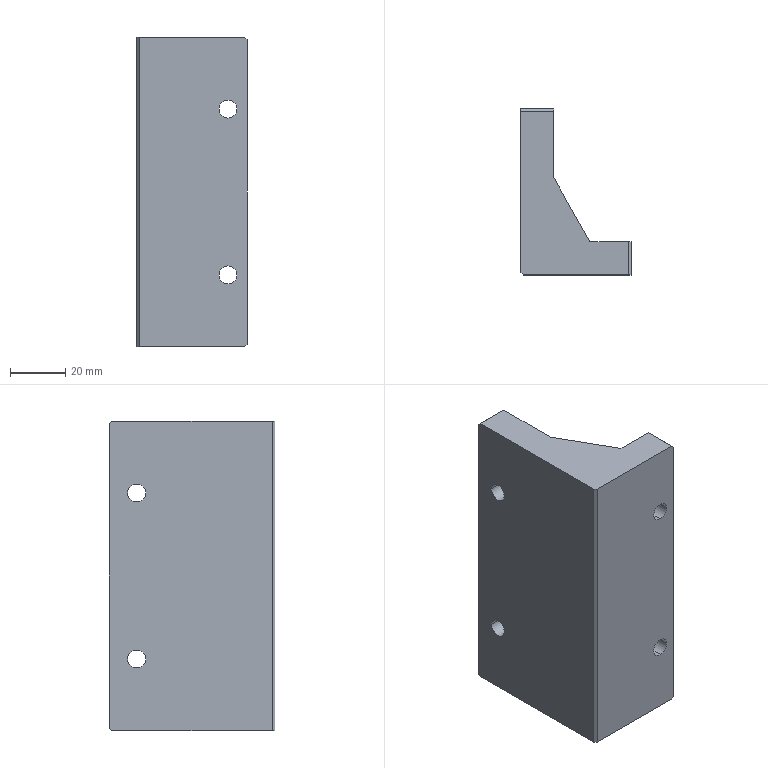Part | NX | features BREP 1 | 1 solid | 34 faces | box 40 x 60 x 112 mm | volume 133076 mm3 | cylinder 14 | plane 14 | cone 6 | commonest cylinder face diameters 6.5 x8 3.3 x6
STEP:
#1=CARTESIAN_POINT('',(9.65,10.,10.1));
#2=VERTEX_POINT('',#1);
#3=CARTESIAN_POINT('',(6.35,10.,10.1));
#4=VERTEX_POINT('',#3);
#5=CARTESIAN_POINT('',(8.,10.,10.1));
#6=DIRECTION('',(0.,0.,-1.));
#7=DIRECTION('',(-1.,0.,0.));
#8=AXIS2_PLACEMENT_3D('',#5,#6,#7);
#9=CIRCLE('',#8,1.65);
#10=EDGE_CURVE('',#2,#4,#9,.T.);
#11=ORIENTED_EDGE('',*,*,#10,.F.);
#12=CARTESIAN_POINT('',(9.65,10.,0.));
#13=VERTEX_POINT('',#12);
#14=CARTESIAN_POINT('',(9.65,10.,0.));
#15=DIRECTION('',(0.,0.,-1.));
#16=VECTOR('',#15,1000.);
#17=LINE('',#14,#16);
#18=EDGE_CURVE('',#2,#13,#17,.T.);
#19=ORIENTED_EDGE('',*,*,#18,.T.);
#20=CARTESIAN_POINT('',(6.35,10.,0.));
#21=VERTEX_POINT('',#20);
#22=CARTESIAN_POINT('',(8.,10.,0.));
#23=DIRECTION('',(0.,0.,-1.));
#24=DIRECTION('',(-1.,0.,0.));
#25=AXIS2_PLACEMENT_3D('',#22,#23,#24);
#26=CIRCLE('',#25,1.65);
#27=EDGE_CURVE('',#13,#21,#26,.T.);
#28=ORIENTED_EDGE('',*,*,#27,.T.);
#29=CARTESIAN_POINT('',(6.35,10.,0.));
#30=DIRECTION('',(0.,0.,-1.));
#31=VECTOR('',#30,1000.);
#32=LINE('',#29,#31);
#33=EDGE_CURVE('',#4,#21,#32,.T.);
#34=ORIENTED_EDGE('',*,*,#33,.F.);
#35=EDGE_LOOP('',(#11,#19,#28,#34));
#36=FACE_BOUND('',#35,.T.);
#37=CARTESIAN_POINT('',(8.,10.,0.));
#38=DIRECTION('',(0.,0.,-1.));
#39=DIRECTION('',(-1.,0.,0.));
#40=AXIS2_PLACEMENT_3D('',#37,#38,#39);
#41=CYLINDRICAL_SURFACE('',#40,1.65);
#42=ADVANCED_FACE('',(#36),#41,.F.);
#43=CARTESIAN_POINT('',(8.,10.,11.091));
#44=VERTEX_POINT('',#43);
#45=CARTESIAN_POINT('',(6.35,10.,10.1));
#46=DIRECTION('',(-0.8572,0.,-0.515));
#47=VECTOR('',#46,1000.);
#48=LINE('',#45,#47);
#49=EDGE_CURVE('',#44,#4,#48,.T.);
#50=ORIENTED_EDGE('',*,*,#49,.F.);
#51=CARTESIAN_POINT('',(9.65,10.,10.1));
#52=DIRECTION('',(0.8572,0.,-0.515));
#53=VECTOR('',#52,1000.);
#54=LINE('',#51,#53);
#55=EDGE_CURVE('',#44,#2,#54,.T.);
#56=ORIENTED_EDGE('',*,*,#55,.T.);
#57=ORIENTED_EDGE('',*,*,#10,.T.);
#58=EDGE_LOOP('',(#50,#56,#57));
#59=FACE_BOUND('',#58,.T.);
#60=CARTESIAN_POINT('',(8.,10.,10.1));
#61=DIRECTION('',(0.,0.,-1.));
#62=DIRECTION('',(-1.,0.,0.));
#63=AXIS2_PLACEMENT_3D('',#60,#61,#62);
#64=CONICAL_SURFACE('',#63,1.65,1.03);
#65=ADVANCED_FACE('',(#59),#64,.F.);
#66=CARTESIAN_POINT('',(8.,49.9,94.35));
#67=VERTEX_POINT('',#66);
#68=CARTESIAN_POINT('',(8.,49.9,97.65));
#69=VERTEX_POINT('',#68);
#70=CARTESIAN_POINT('',(8.,49.9,96.));
#71=DIRECTION('',(0.,1.,0.));
#72=DIRECTION('',(0.,0.,1.));
#73=AXIS2_PLACEMENT_3D('',#70,#71,#72);
#74=CIRCLE('',#73,1.65);
#75=EDGE_CURVE('',#67,#69,#74,.T.);
#76=ORIENTED_EDGE('',*,*,#75,.F.);
#77=CARTESIAN_POINT('',(8.,60.,94.35));
#78=VERTEX_POINT('',#77);
#79=CARTESIAN_POINT('',(8.,60.,94.35));
#80=DIRECTION('',(0.,1.,0.));
#81=VECTOR('',#80,1000.);
#82=LINE('',#79,#81);
#83=EDGE_CURVE('',#78,#67,#82,.F.);
#84=ORIENTED_EDGE('',*,*,#83,.F.);
#85=CARTESIAN_POINT('',(8.,60.,97.65));
#86=VERTEX_POINT('',#85);
#87=CARTESIAN_POINT('',(8.,60.,96.));
#88=DIRECTION('',(0.,1.,0.));
#89=DIRECTION('',(0.,0.,1.));
#90=AXIS2_PLACEMENT_3D('',#87,#88,#89);
#91=CIRCLE('',#90,1.65);
#92=EDGE_CURVE('',#78,#86,#91,.T.);
#93=ORIENTED_EDGE('',*,*,#92,.T.);
#94=CARTESIAN_POINT('',(8.,60.,97.65));
#95=DIRECTION('',(0.,1.,0.));
#96=VECTOR('',#95,1000.);
#97=LINE('',#94,#96);
#98=EDGE_CURVE('',#86,#69,#97,.F.);
#99=ORIENTED_EDGE('',*,*,#98,.T.);
#100=EDGE_LOOP('',(#76,#84,#93,#99));
#101=FACE_BOUND('',#100,.T.);
#102=CARTESIAN_POINT('',(8.,60.,96.));
#103=DIRECTION('',(0.,1.,0.));
#104=DIRECTION('',(0.,0.,1.));
#105=AXIS2_PLACEMENT_3D('',#102,#103,#104);
#106=CYLINDRICAL_SURFACE('',#105,1.65);
#107=ADVANCED_FACE('',(#101),#106,.F.);
#108=CARTESIAN_POINT('',(8.,48.909,96.));
#109=VERTEX_POINT('',#108);
#110=CARTESIAN_POINT('',(8.,49.9,97.65));
#111=DIRECTION('',(0.,0.515,0.8572));
#112=VECTOR('',#111,1000.);
#113=LINE('',#110,#112);
#114=EDGE_CURVE('',#69,#109,#113,.F.);
#115=ORIENTED_EDGE('',*,*,#114,.T.);
#116=CARTESIAN_POINT('',(8.,49.9,94.35));
#117=DIRECTION('',(0.,0.515,-0.8572));
#118=VECTOR('',#117,1000.);
#119=LINE('',#116,#118);
#120=EDGE_CURVE('',#67,#109,#119,.F.);
#121=ORIENTED_EDGE('',*,*,#120,.F.);
#122=ORIENTED_EDGE('',*,*,#75,.T.);
#123=EDGE_LOOP('',(#115,#121,#122));
#124=FACE_BOUND('',#123,.T.);
#125=CARTESIAN_POINT('',(8.,49.9,96.));
#126=DIRECTION('',(0.,1.,0.));
#127=DIRECTION('',(0.,0.,1.));
#128=AXIS2_PLACEMENT_3D('',#125,#126,#127);
#129=CONICAL_SURFACE('',#128,1.65,1.03);
#130=ADVANCED_FACE('',(#124),#129,.F.);
#131=CARTESIAN_POINT('',(8.,49.9,14.35));
#132=VERTEX_POINT('',#131);
#133=CARTESIAN_POINT('',(8.,49.9,17.65));
#134=VERTEX_POINT('',#133);
#135=CARTESIAN_POINT('',(8.,49.9,16.));
#136=DIRECTION('',(0.,1.,0.));
#137=DIRECTION('',(0.,0.,1.));
#138=AXIS2_PLACEMENT_3D('',#135,#136,#137);
#139=CIRCLE('',#138,1.65);
#140=EDGE_CURVE('',#132,#134,#139,.T.);
#141=ORIENTED_EDGE('',*,*,#140,.F.);
#142=CARTESIAN_POINT('',(8.,60.,14.35));
#143=VERTEX_POINT('',#142);
#144=CARTESIAN_POINT('',(8.,60.,14.35));
#145=DIRECTION('',(0.,1.,0.));
#146=VECTOR('',#145,1000.);
#147=LINE('',#144,#146);
#148=EDGE_CURVE('',#143,#132,#147,.F.);
#149=ORIENTED_EDGE('',*,*,#148,.F.);
#150=CARTESIAN_POINT('',(8.,60.,17.65));
#151=VERTEX_POINT('',#150);
#152=CARTESIAN_POINT('',(8.,60.,16.));
#153=DIRECTION('',(0.,1.,0.));
#154=DIRECTION('',(0.,0.,1.));
#155=AXIS2_PLACEMENT_3D('',#152,#153,#154);
#156=CIRCLE('',#155,1.65);
#157=EDGE_CURVE('',#143,#151,#156,.T.);
#158=ORIENTED_EDGE('',*,*,#157,.T.);
#159=CARTESIAN_POINT('',(8.,60.,17.65));
#160=DIRECTION('',(0.,1.,0.));
#161=VECTOR('',#160,1000.);
#162=LINE('',#159,#161);
#163=EDGE_CURVE('',#151,#134,#162,.F.);
#164=ORIENTED_EDGE('',*,*,#163,.T.);
#165=EDGE_LOOP('',(#141,#149,#158,#164));
#166=FACE_BOUND('',#165,.T.);
#167=CARTESIAN_POINT('',(8.,60.,16.));
#168=DIRECTION('',(0.,1.,0.));
#169=DIRECTION('',(0.,0.,1.));
#170=AXIS2_PLACEMENT_3D('',#167,#168,#169);
#171=CYLINDRICAL_SURFACE('',#170,1.65);
#172=ADVANCED_FACE('',(#166),#171,.F.);
#173=CARTESIAN_POINT('',(8.,48.909,16.));
#174=VERTEX_POINT('',#173);
#175=CARTESIAN_POINT('',(8.,49.9,17.65));
#176=DIRECTION('',(0.,0.515,0.8572));
#177=VECTOR('',#176,1000.);
#178=LINE('',#175,#177);
#179=EDGE_CURVE('',#134,#174,#178,.F.);
#180=ORIENTED_EDGE('',*,*,#179,.T.);
#181=CARTESIAN_POINT('',(8.,49.9,14.35));
#182=DIRECTION('',(0.,0.515,-0.8572));
#183=VECTOR('',#182,1000.);
#184=LINE('',#181,#183);
#185=EDGE_CURVE('',#132,#174,#184,.F.);
#186=ORIENTED_EDGE('',*,*,#185,.F.);
#187=ORIENTED_EDGE('',*,*,#140,.T.);
#188=EDGE_LOOP('',(#180,#186,#187));
#189=FACE_BOUND('',#188,.T.);
#190=CARTESIAN_POINT('',(8.,49.9,16.));
#191=DIRECTION('',(0.,1.,0.));
#192=DIRECTION('',(0.,0.,1.));
#193=AXIS2_PLACEMENT_3D('',#190,#191,#192);
#194=CONICAL_SURFACE('',#193,1.65,1.03);
#195=ADVANCED_FACE('',(#189),#194,.F.);
#196=CARTESIAN_POINT('',(0.,46.75,86.));
#197=VERTEX_POINT('',#196);
#198=CARTESIAN_POINT('',(0.,53.25,86.));
#199=VERTEX_POINT('',#198);
#200=CARTESIAN_POINT('',(0.,50.,86.));
#201=DIRECTION('',(1.,0.,0.));
#202=DIRECTION('',(0.,0.,-1.));
#203=AXIS2_PLACEMENT_3D('',#200,#201,#202);
#204=CIRCLE('',#203,3.25);
#205=EDGE_CURVE('',#197,#199,#204,.T.);
#206=ORIENTED_EDGE('',*,*,#205,.F.);
#207=CARTESIAN_POINT('',(12.,46.75,86.));
#208=VERTEX_POINT('',#207);
#209=CARTESIAN_POINT('',(-18.,46.75,86.));
#210=DIRECTION('',(1.,0.,0.));
#211=VECTOR('',#210,1000.);
#212=LINE('',#209,#211);
#213=EDGE_CURVE('',#208,#197,#212,.F.);
#214=ORIENTED_EDGE('',*,*,#213,.F.);
#215=CARTESIAN_POINT('',(12.,53.25,86.));
#216=VERTEX_POINT('',#215);
#217=CARTESIAN_POINT('',(12.,50.,86.));
#218=DIRECTION('',(1.,0.,0.));
#219=DIRECTION('',(0.,1.,0.));
#220=AXIS2_PLACEMENT_3D('',#217,#218,#219);
#221=CIRCLE('',#220,3.25);
#222=EDGE_CURVE('',#208,#216,#221,.T.);
#223=ORIENTED_EDGE('',*,*,#222,.T.);
#224=CARTESIAN_POINT('',(-18.,53.25,86.));
#225=DIRECTION('',(1.,0.,0.));
#226=VECTOR('',#225,1000.);
#227=LINE('',#224,#226);
#228=EDGE_CURVE('',#216,#199,#227,.F.);
#229=ORIENTED_EDGE('',*,*,#228,.T.);
#230=EDGE_LOOP('',(#206,#214,#223,#229));
#231=FACE_BOUND('',#230,.T.);
#232=CARTESIAN_POINT('',(-18.,50.,86.));
#233=DIRECTION('',(1.,0.,0.));
#234=DIRECTION('',(0.,1.,0.));
#235=AXIS2_PLACEMENT_3D('',#232,#233,#234);
#236=CYLINDRICAL_SURFACE('',#235,3.25);
#237=ADVANCED_FACE('',(#231),#236,.F.);
#238=CARTESIAN_POINT('',(0.,46.75,26.));
#239=VERTEX_POINT('',#238);
#240=CARTESIAN_POINT('',(0.,53.25,26.));
#241=VERTEX_POINT('',#240);
#242=CARTESIAN_POINT('',(0.,50.,26.));
#243=DIRECTION('',(1.,0.,0.));
#244=DIRECTION('',(0.,0.,-1.));
#245=AXIS2_PLACEMENT_3D('',#242,#243,#244);
#246=CIRCLE('',#245,3.25);
#247=EDGE_CURVE('',#239,#241,#246,.T.);
#248=ORIENTED_EDGE('',*,*,#247,.F.);
#249=CARTESIAN_POINT('',(12.,46.75,26.));
#250=VERTEX_POINT('',#249);
#251=CARTESIAN_POINT('',(-18.,46.75,26.));
#252=DIRECTION('',(1.,0.,0.));
#253=VECTOR('',#252,1000.);
#254=LINE('',#251,#253);
#255=EDGE_CURVE('',#250,#239,#254,.F.);
#256=ORIENTED_EDGE('',*,*,#255,.F.);
#257=CARTESIAN_POINT('',(12.,53.25,26.));
#258=VERTEX_POINT('',#257);
#259=CARTESIAN_POINT('',(12.,50.,26.));
#260=DIRECTION('',(1.,0.,0.));
#261=DIRECTION('',(0.,1.,0.));
#262=AXIS2_PLACEMENT_3D('',#259,#260,#261);
#263=CIRCLE('',#262,3.25);
#264=EDGE_CURVE('',#250,#258,#263,.T.);
#265=ORIENTED_EDGE('',*,*,#264,.T.);
#266=CARTESIAN_POINT('',(-18.,53.25,26.));
#267=DIRECTION('',(1.,0.,0.));
#268=VECTOR('',#267,1000.);
#269=LINE('',#266,#268);
#270=EDGE_CURVE('',#258,#241,#269,.F.);
#271=ORIENTED_EDGE('',*,*,#270,.T.);
#272=EDGE_LOOP('',(#248,#256,#265,#271));
#273=FACE_BOUND('',#272,.T.);
#274=CARTESIAN_POINT('',(-18.,50.,26.));
#275=DIRECTION('',(1.,0.,0.));
#276=DIRECTION('',(0.,1.,0.));
#277=AXIS2_PLACEMENT_3D('',#274,#275,#276);
#278=CYLINDRICAL_SURFACE('',#277,3.25);
#279=ADVANCED_FACE('',(#273),#278,.F.);
#280=CARTESIAN_POINT('',(33.,0.,22.75));
#281=VERTEX_POINT('',#280);
#282=CARTESIAN_POINT('',(33.,0.,29.25));
#283=VERTEX_POINT('',#282);
#284=CARTESIAN_POINT('',(33.,0.,26.));
#285=DIRECTION('',(0.,1.,0.));
#286=DIRECTION('',(0.,0.,1.));
#287=AXIS2_PLACEMENT_3D('',#284,#285,#286);
#288=CIRCLE('',#287,3.25);
#289=EDGE_CURVE('',#281,#283,#288,.T.);
#290=ORIENTED_EDGE('',*,*,#289,.F.);
#291=CARTESIAN_POINT('',(33.,12.,22.75));
#292=VERTEX_POINT('',#291);
#293=CARTESIAN_POINT('',(33.,12.,22.75));
#294=DIRECTION('',(0.,1.,0.));
#295=VECTOR('',#294,1000.);
#296=LINE('',#293,#295);
#297=EDGE_CURVE('',#292,#281,#296,.F.);
#298=ORIENTED_EDGE('',*,*,#297,.F.);
#299=CARTESIAN_POINT('',(33.,12.,29.25));
#300=VERTEX_POINT('',#299);
#301=CARTESIAN_POINT('',(33.,12.,26.));
#302=DIRECTION('',(0.,1.,0.));
#303=DIRECTION('',(0.,0.,1.));
#304=AXIS2_PLACEMENT_3D('',#301,#302,#303);
#305=CIRCLE('',#304,3.25);
#306=EDGE_CURVE('',#292,#300,#305,.T.);
#307=ORIENTED_EDGE('',*,*,#306,.T.);
#308=CARTESIAN_POINT('',(33.,12.,29.25));
#309=DIRECTION('',(0.,1.,0.));
#310=VECTOR('',#309,1000.);
#311=LINE('',#308,#310);
#312=EDGE_CURVE('',#300,#283,#311,.F.);
#313=ORIENTED_EDGE('',*,*,#312,.T.);
#314=EDGE_LOOP('',(#290,#298,#307,#313));
#315=FACE_BOUND('',#314,.T.);
#316=CARTESIAN_POINT('',(33.,12.,26.));
#317=DIRECTION('',(0.,1.,0.));
#318=DIRECTION('',(0.,0.,1.));
#319=AXIS2_PLACEMENT_3D('',#316,#317,#318);
#320=CYLINDRICAL_SURFACE('',#319,3.25);
#321=ADVANCED_FACE('',(#315),#320,.F.);
#322=CARTESIAN_POINT('',(33.,0.,82.75));
#323=VERTEX_POINT('',#322);
#324=CARTESIAN_POINT('',(33.,0.,89.25));
#325=VERTEX_POINT('',#324);
#326=CARTESIAN_POINT('',(33.,0.,86.));
#327=DIRECTION('',(0.,1.,0.));
#328=DIRECTION('',(0.,0.,1.));
#329=AXIS2_PLACEMENT_3D('',#326,#327,#328);
#330=CIRCLE('',#329,3.25);
#331=EDGE_CURVE('',#323,#325,#330,.T.);
#332=ORIENTED_EDGE('',*,*,#331,.F.);
#333=CARTESIAN_POINT('',(33.,12.,82.75));
#334=VERTEX_POINT('',#333);
#335=CARTESIAN_POINT('',(33.,12.,82.75));
#336=DIRECTION('',(0.,1.,0.));
#337=VECTOR('',#336,1000.);
#338=LINE('',#335,#337);
#339=EDGE_CURVE('',#334,#323,#338,.F.);
#340=ORIENTED_EDGE('',*,*,#339,.F.);
#341=CARTESIAN_POINT('',(33.,12.,89.25));
#342=VERTEX_POINT('',#341);
#343=CARTESIAN_POINT('',(33.,12.,86.));
#344=DIRECTION('',(0.,1.,0.));
#345=DIRECTION('',(0.,0.,1.));
#346=AXIS2_PLACEMENT_3D('',#343,#344,#345);
#347=CIRCLE('',#346,3.25);
#348=EDGE_CURVE('',#334,#342,#347,.T.);
#349=ORIENTED_EDGE('',*,*,#348,.T.);
#350=CARTESIAN_POINT('',(33.,12.,89.25));
#351=DIRECTION('',(0.,1.,0.));
#352=VECTOR('',#351,1000.);
#353=LINE('',#350,#352);
#354=EDGE_CURVE('',#342,#325,#353,.F.);
#355=ORIENTED_EDGE('',*,*,#354,.T.);
#356=EDGE_LOOP('',(#332,#340,#349,#355));
#357=FACE_BOUND('',#356,.T.);
#358=CARTESIAN_POINT('',(33.,12.,86.));
#359=DIRECTION('',(0.,1.,0.));
#360=DIRECTION('',(0.,0.,1.));
#361=AXIS2_PLACEMENT_3D('',#358,#359,#360);
#362=CYLINDRICAL_SURFACE('',#361,3.25);
#363=ADVANCED_FACE('',(#357),#362,.F.);
#364=CARTESIAN_POINT('',(1.,0.,112.));
#365=VERTEX_POINT('',#364);
#366=CARTESIAN_POINT('',(39.,0.,112.));
#367=VERTEX_POINT('',#366);
#368=CARTESIAN_POINT('',(40.,0.,112.));
#369=DIRECTION('',(1.,0.,0.));
#370=VECTOR('',#369,1000.);
#371=LINE('',#368,#370);
#372=EDGE_CURVE('',#365,#367,#371,.T.);
#373=ORIENTED_EDGE('',*,*,#372,.F.);
#374=CARTESIAN_POINT('',(1.,0.,0.));
#375=VERTEX_POINT('',#374);
#376=CARTESIAN_POINT('',(1.,0.,112.));
#377=DIRECTION('',(0.,0.,-1.));
#378=VECTOR('',#377,1000.);
#379=LINE('',#376,#378);
#380=EDGE_CURVE('',#365,#375,#379,.T.);
#381=ORIENTED_EDGE('',*,*,#380,.T.);
#382=CARTESIAN_POINT('',(39.,0.,0.));
#383=VERTEX_POINT('',#382);
#384=CARTESIAN_POINT('',(40.,0.,0.));
#385=DIRECTION('',(1.,0.,0.));
#386=VECTOR('',#385,1000.);
#387=LINE('',#384,#386);
#388=EDGE_CURVE('',#375,#383,#387,.T.);
#389=ORIENTED_EDGE('',*,*,#388,.T.);
#390=CARTESIAN_POINT('',(40.,0.,1.));
#391=VERTEX_POINT('',#390);
#392=CARTESIAN_POINT('',(40.,0.,1.));
#393=DIRECTION('',(0.7071,0.,0.7071));
#394=VECTOR('',#393,1000.);
#395=LINE('',#392,#394);
#396=EDGE_CURVE('',#383,#391,#395,.T.);
#397=ORIENTED_EDGE('',*,*,#396,.T.);
#398=CARTESIAN_POINT('',(40.,0.,111.));
#399=VERTEX_POINT('',#398);
#400=CARTESIAN_POINT('',(40.,0.,112.));
#401=DIRECTION('',(0.,0.,-1.));
#402=VECTOR('',#401,1000.);
#403=LINE('',#400,#402);
#404=EDGE_CURVE('',#399,#391,#403,.T.);
#405=ORIENTED_EDGE('',*,*,#404,.F.);
#406=CARTESIAN_POINT('',(39.,0.,112.));
#407=DIRECTION('',(-0.7071,0.,0.7071));
#408=VECTOR('',#407,1000.);
#409=LINE('',#406,#408);
#410=EDGE_CURVE('',#399,#367,#409,.T.);
#411=ORIENTED_EDGE('',*,*,#410,.T.);
#412=EDGE_LOOP('',(#373,#381,#389,#397,#405,#411));
#413=FACE_BOUND('',#412,.T.);
#414=CARTESIAN_POINT('',(33.,0.,26.));
#415=DIRECTION('',(0.,1.,0.));
#416=DIRECTION('',(0.,0.,1.));
#417=AXIS2_PLACEMENT_3D('',#414,#415,#416);
#418=CIRCLE('',#417,3.25);
#419=EDGE_CURVE('',#283,#281,#418,.T.);
#420=ORIENTED_EDGE('',*,*,#419,.T.);
#421=ORIENTED_EDGE('',*,*,#289,.T.);
#422=EDGE_LOOP('',(#420,#421));
#423=FACE_BOUND('',#422,.T.);
#424=CARTESIAN_POINT('',(33.,0.,86.));
#425=DIRECTION('',(0.,1.,0.));
#426=DIRECTION('',(0.,0.,1.));
#427=AXIS2_PLACEMENT_3D('',#424,#425,#426);
#428=CIRCLE('',#427,3.25);
#429=EDGE_CURVE('',#325,#323,#428,.T.);
#430=ORIENTED_EDGE('',*,*,#429,.T.);
#431=ORIENTED_EDGE('',*,*,#331,.T.);
#432=EDGE_LOOP('',(#430,#431));
#433=FACE_BOUND('',#432,.T.);
#434=CARTESIAN_POINT('',(40.,0.,112.));
#435=DIRECTION('',(0.,1.,0.));
#436=DIRECTION('',(1.,0.,0.));
#437=AXIS2_PLACEMENT_3D('',#434,#435,#436);
#438=PLANE('',#437);
#439=ADVANCED_FACE('',(#413,#423,#433),#438,.F.);
#440=ORIENTED_EDGE('',*,*,#404,.T.);
#441=CARTESIAN_POINT('',(40.,12.,1.));
#442=VERTEX_POINT('',#441);
#443=CARTESIAN_POINT('',(40.,12.,1.));
#444=DIRECTION('',(0.,1.,0.));
#445=VECTOR('',#444,1000.);
#446=LINE('',#443,#445);
#447=EDGE_CURVE('',#391,#442,#446,.T.);
#448=ORIENTED_EDGE('',*,*,#447,.T.);
#449=CARTESIAN_POINT('',(40.,12.,111.));
#450=VERTEX_POINT('',#449);
#451=CARTESIAN_POINT('',(40.,12.,112.));
#452=DIRECTION('',(0.,0.,-1.));
#453=VECTOR('',#452,1000.);
#454=LINE('',#451,#453);
#455=EDGE_CURVE('',#450,#442,#454,.T.);
#456=ORIENTED_EDGE('',*,*,#455,.F.);
#457=CARTESIAN_POINT('',(40.,12.,111.));
#458=DIRECTION('',(0.,-1.,0.));
#459=VECTOR('',#458,1000.);
#460=LINE('',#457,#459);
#461=EDGE_CURVE('',#450,#399,#460,.T.);
#462=ORIENTED_EDGE('',*,*,#461,.T.);
#463=EDGE_LOOP('',(#440,#448,#456,#462));
#464=FACE_BOUND('',#463,.T.);
#465=CARTESIAN_POINT('',(40.,12.,112.));
#466=DIRECTION('',(-1.,0.,0.));
#467=DIRECTION('',(0.,0.,1.));
#468=AXIS2_PLACEMENT_3D('',#465,#466,#467);
#469=PLANE('',#468);
#470=ADVANCED_FACE('',(#464),#469,.F.);
#471=ORIENTED_EDGE('',*,*,#455,.T.);
#472=CARTESIAN_POINT('',(39.,12.,0.));
#473=VERTEX_POINT('',#472);
#474=CARTESIAN_POINT('',(40.,12.,1.));
#475=DIRECTION('',(-0.7071,0.,-0.7071));
#476=VECTOR('',#475,1000.);
#477=LINE('',#474,#476);
#478=EDGE_CURVE('',#442,#473,#477,.T.);
#479=ORIENTED_EDGE('',*,*,#478,.T.);
#480=CARTESIAN_POINT('',(25.,12.,0.));
#481=VERTEX_POINT('',#480);
#482=CARTESIAN_POINT('',(25.,12.,0.));
#483=DIRECTION('',(-1.,0.,0.));
#484=VECTOR('',#483,1000.);
#485=LINE('',#482,#484);
#486=EDGE_CURVE('',#473,#481,#485,.T.);
#487=ORIENTED_EDGE('',*,*,#486,.T.);
#488=CARTESIAN_POINT('',(25.,12.,112.));
#489=VERTEX_POINT('',#488);
#490=CARTESIAN_POINT('',(25.,12.,112.));
#491=DIRECTION('',(0.,0.,-1.));
#492=VECTOR('',#491,1000.);
#493=LINE('',#490,#492);
#494=EDGE_CURVE('',#489,#481,#493,.T.);
#495=ORIENTED_EDGE('',*,*,#494,.F.);
#496=CARTESIAN_POINT('',(39.,12.,112.));
#497=VERTEX_POINT('',#496);
#498=CARTESIAN_POINT('',(25.,12.,112.));
#499=DIRECTION('',(-1.,0.,0.));
#500=VECTOR('',#499,1000.);
#501=LINE('',#498,#500);
#502=EDGE_CURVE('',#497,#489,#501,.T.);
#503=ORIENTED_EDGE('',*,*,#502,.F.);
#504=CARTESIAN_POINT('',(39.,12.,112.));
#505=DIRECTION('',(0.7071,0.,-0.7071));
#506=VECTOR('',#505,1000.);
#507=LINE('',#504,#506);
#508=EDGE_CURVE('',#497,#450,#507,.T.);
#509=ORIENTED_EDGE('',*,*,#508,.T.);
#510=EDGE_LOOP('',(#471,#479,#487,#495,#503,#509));
#511=FACE_BOUND('',#510,.T.);
#512=CARTESIAN_POINT('',(33.,12.,26.));
#513=DIRECTION('',(0.,1.,0.));
#514=DIRECTION('',(0.,0.,1.));
#515=AXIS2_PLACEMENT_3D('',#512,#513,#514);
#516=CIRCLE('',#515,3.25);
#517=EDGE_CURVE('',#300,#292,#516,.T.);
#518=ORIENTED_EDGE('',*,*,#517,.F.);
#519=ORIENTED_EDGE('',*,*,#306,.F.);
#520=EDGE_LOOP('',(#518,#519));
#521=FACE_BOUND('',#520,.T.);
#522=CARTESIAN_POINT('',(33.,12.,86.));
#523=DIRECTION('',(0.,1.,0.));
#524=DIRECTION('',(0.,0.,1.));
#525=AXIS2_PLACEMENT_3D('',#522,#523,#524);
#526=CIRCLE('',#525,3.25);
#527=EDGE_CURVE('',#342,#334,#526,.T.);
#528=ORIENTED_EDGE('',*,*,#527,.F.);
#529=ORIENTED_EDGE('',*,*,#348,.F.);
#530=EDGE_LOOP('',(#528,#529));
#531=FACE_BOUND('',#530,.T.);
#532=CARTESIAN_POINT('',(25.,12.,112.));
#533=DIRECTION('',(0.,-1.,0.));
#534=DIRECTION('',(0.,0.,-1.));
#535=AXIS2_PLACEMENT_3D('',#532,#533,#534);
#536=PLANE('',#535);
#537=ADVANCED_FACE('',(#511,#521,#531),#536,.F.);
#538=CARTESIAN_POINT('',(12.,35.,0.));
#539=VERTEX_POINT('',#538);
#540=CARTESIAN_POINT('',(12.,35.,0.));
#541=DIRECTION('',(-0.4921,0.8706,0.));
#542=VECTOR('',#541,1000.);
#543=LINE('',#540,#542);
#544=EDGE_CURVE('',#481,#539,#543,.T.);
#545=ORIENTED_EDGE('',*,*,#544,.T.);
#546=CARTESIAN_POINT('',(12.,35.,112.));
#547=VERTEX_POINT('',#546);
#548=CARTESIAN_POINT('',(12.,35.,112.));
#549=DIRECTION('',(0.,0.,-1.));
#550=VECTOR('',#549,1000.);
#551=LINE('',#548,#550);
#552=EDGE_CURVE('',#547,#539,#551,.T.);
#553=ORIENTED_EDGE('',*,*,#552,.F.);
#554=CARTESIAN_POINT('',(12.,35.,112.));
#555=DIRECTION('',(-0.4921,0.8706,0.));
#556=VECTOR('',#555,1000.);
#557=LINE('',#554,#556);
#558=EDGE_CURVE('',#489,#547,#557,.T.);
#559=ORIENTED_EDGE('',*,*,#558,.F.);
#560=ORIENTED_EDGE('',*,*,#494,.T.);
#561=EDGE_LOOP('',(#545,#553,#559,#560));
#562=FACE_BOUND('',#561,.T.);
#563=CARTESIAN_POINT('',(12.,35.,112.));
#564=DIRECTION('',(-0.8706,-0.4921,0.));
#565=DIRECTION('',(-0.4921,0.8706,0.));
#566=AXIS2_PLACEMENT_3D('',#563,#564,#565);
#567=PLANE('',#566);
#568=ADVANCED_FACE('',(#562),#567,.F.);
#569=CARTESIAN_POINT('',(12.,60.,111.));
#570=VERTEX_POINT('',#569);
#571=CARTESIAN_POINT('',(12.,60.,1.));
#572=VERTEX_POINT('',#571);
#573=CARTESIAN_POINT('',(12.,60.,112.));
#574=DIRECTION('',(0.,0.,-1.));
#575=VECTOR('',#574,1000.);
#576=LINE('',#573,#575);
#577=EDGE_CURVE('',#570,#572,#576,.T.);
#578=ORIENTED_EDGE('',*,*,#577,.F.);
#579=CARTESIAN_POINT('',(12.,59.,112.));
#580=VERTEX_POINT('',#579);
#581=CARTESIAN_POINT('',(12.,59.,112.));
#582=DIRECTION('',(0.,-0.7071,0.7071));
#583=VECTOR('',#582,1000.);
#584=LINE('',#581,#583);
#585=EDGE_CURVE('',#570,#580,#584,.T.);
#586=ORIENTED_EDGE('',*,*,#585,.T.);
#587=CARTESIAN_POINT('',(12.,60.,112.));
#588=DIRECTION('',(0.,1.,0.));
#589=VECTOR('',#588,1000.);
#590=LINE('',#587,#589);
#591=EDGE_CURVE('',#547,#580,#590,.T.);
#592=ORIENTED_EDGE('',*,*,#591,.F.);
#593=ORIENTED_EDGE('',*,*,#552,.T.);
#594=CARTESIAN_POINT('',(12.,59.,0.));
#595=VERTEX_POINT('',#594);
#596=CARTESIAN_POINT('',(12.,60.,0.));
#597=DIRECTION('',(0.,1.,0.));
#598=VECTOR('',#597,1000.);
#599=LINE('',#596,#598);
#600=EDGE_CURVE('',#539,#595,#599,.T.);
#601=ORIENTED_EDGE('',*,*,#600,.T.);
#602=CARTESIAN_POINT('',(12.,60.,1.));
#603=DIRECTION('',(0.,0.7071,0.7071));
#604=VECTOR('',#603,1000.);
#605=LINE('',#602,#604);
#606=EDGE_CURVE('',#595,#572,#605,.T.);
#607=ORIENTED_EDGE('',*,*,#606,.T.);
#608=EDGE_LOOP('',(#578,#586,#592,#593,#601,#607));
#609=FACE_BOUND('',#608,.T.);
#610=CARTESIAN_POINT('',(12.,50.,86.));
#611=DIRECTION('',(1.,0.,0.));
#612=DIRECTION('',(0.,1.,0.));
#613=AXIS2_PLACEMENT_3D('',#610,#611,#612);
#614=CIRCLE('',#613,3.25);
#615=EDGE_CURVE('',#216,#208,#614,.T.);
#616=ORIENTED_EDGE('',*,*,#615,.F.);
#617=ORIENTED_EDGE('',*,*,#222,.F.);
#618=EDGE_LOOP('',(#616,#617));
#619=FACE_BOUND('',#618,.T.);
#620=CARTESIAN_POINT('',(12.,50.,26.));
#621=DIRECTION('',(1.,0.,0.));
#622=DIRECTION('',(0.,1.,0.));
#623=AXIS2_PLACEMENT_3D('',#620,#621,#622);
#624=CIRCLE('',#623,3.25);
#625=EDGE_CURVE('',#258,#250,#624,.T.);
#626=ORIENTED_EDGE('',*,*,#625,.F.);
#627=ORIENTED_EDGE('',*,*,#264,.F.);
#628=EDGE_LOOP('',(#626,#627));
#629=FACE_BOUND('',#628,.T.);
#630=CARTESIAN_POINT('',(12.,60.,112.));
#631=DIRECTION('',(-1.,0.,0.));
#632=DIRECTION('',(0.,1.,0.));
#633=AXIS2_PLACEMENT_3D('',#630,#631,#632);
#634=PLANE('',#633);
#635=ADVANCED_FACE('',(#609,#619,#629),#634,.F.);
#636=CARTESIAN_POINT('',(0.,60.,111.));
#637=VERTEX_POINT('',#636);
#638=CARTESIAN_POINT('',(0.,60.,1.));
#639=VERTEX_POINT('',#638);
#640=CARTESIAN_POINT('',(0.,60.,112.));
#641=DIRECTION('',(0.,0.,-1.));
#642=VECTOR('',#641,1000.);
#643=LINE('',#640,#642);
#644=EDGE_CURVE('',#637,#639,#643,.T.);
#645=ORIENTED_EDGE('',*,*,#644,.F.);
#646=CARTESIAN_POINT('',(0.,60.,111.));
#647=DIRECTION('',(1.,0.,0.));
#648=VECTOR('',#647,1000.);
#649=LINE('',#646,#648);
#650=EDGE_CURVE('',#637,#570,#649,.T.);
#651=ORIENTED_EDGE('',*,*,#650,.T.);
#652=ORIENTED_EDGE('',*,*,#577,.T.);
#653=CARTESIAN_POINT('',(0.,60.,1.));
#654=DIRECTION('',(-1.,0.,0.));
#655=VECTOR('',#654,1000.);
#656=LINE('',#653,#655);
#657=EDGE_CURVE('',#572,#639,#656,.T.);
#658=ORIENTED_EDGE('',*,*,#657,.T.);
#659=EDGE_LOOP('',(#645,#651,#652,#658));
#660=FACE_BOUND('',#659,.T.);
#661=CARTESIAN_POINT('',(8.,60.,96.));
#662=DIRECTION('',(0.,1.,0.));
#663=DIRECTION('',(0.,0.,1.));
#664=AXIS2_PLACEMENT_3D('',#661,#662,#663);
#665=CIRCLE('',#664,1.65);
#666=EDGE_CURVE('',#86,#78,#665,.T.);
#667=ORIENTED_EDGE('',*,*,#666,.F.);
#668=ORIENTED_EDGE('',*,*,#92,.F.);
#669=EDGE_LOOP('',(#667,#668));
#670=FACE_BOUND('',#669,.T.);
#671=CARTESIAN_POINT('',(8.,60.,16.));
#672=DIRECTION('',(0.,1.,0.));
#673=DIRECTION('',(0.,0.,1.));
#674=AXIS2_PLACEMENT_3D('',#671,#672,#673);
#675=CIRCLE('',#674,1.65);
#676=EDGE_CURVE('',#151,#143,#675,.T.);
#677=ORIENTED_EDGE('',*,*,#676,.F.);
#678=ORIENTED_EDGE('',*,*,#157,.F.);
#679=EDGE_LOOP('',(#677,#678));
#680=FACE_BOUND('',#679,.T.);
#681=CARTESIAN_POINT('',(0.,60.,112.));
#682=DIRECTION('',(0.,-1.,0.));
#683=DIRECTION('',(0.,0.,-1.));
#684=AXIS2_PLACEMENT_3D('',#681,#682,#683);
#685=PLANE('',#684);
#686=ADVANCED_FACE('',(#660,#670,#680),#685,.F.);
#687=CARTESIAN_POINT('',(0.,59.,0.));
#688=VERTEX_POINT('',#687);
#689=CARTESIAN_POINT('',(0.,1.,0.));
#690=VERTEX_POINT('',#689);
#691=CARTESIAN_POINT('',(0.,0.,0.));
#692=DIRECTION('',(0.,-1.,0.));
#693=VECTOR('',#692,1000.);
#694=LINE('',#691,#693);
#695=EDGE_CURVE('',#688,#690,#694,.T.);
#696=ORIENTED_EDGE('',*,*,#695,.T.);
#697=CARTESIAN_POINT('',(0.,1.,112.));
#698=VERTEX_POINT('',#697);
#699=CARTESIAN_POINT('',(0.,1.,112.));
#700=DIRECTION('',(0.,0.,1.));
#701=VECTOR('',#700,1000.);
#702=LINE('',#699,#701);
#703=EDGE_CURVE('',#690,#698,#702,.T.);
#704=ORIENTED_EDGE('',*,*,#703,.T.);
#705=CARTESIAN_POINT('',(0.,59.,112.));
#706=VERTEX_POINT('',#705);
#707=CARTESIAN_POINT('',(0.,0.,112.));
#708=DIRECTION('',(0.,-1.,0.));
#709=VECTOR('',#708,1000.);
#710=LINE('',#707,#709);
#711=EDGE_CURVE('',#706,#698,#710,.T.);
#712=ORIENTED_EDGE('',*,*,#711,.F.);
#713=CARTESIAN_POINT('',(0.,59.,112.));
#714=DIRECTION('',(0.,0.7071,-0.7071));
#715=VECTOR('',#714,1000.);
#716=LINE('',#713,#715);
#717=EDGE_CURVE('',#706,#637,#716,.T.);
#718=ORIENTED_EDGE('',*,*,#717,.T.);
#719=ORIENTED_EDGE('',*,*,#644,.T.);
#720=CARTESIAN_POINT('',(0.,60.,1.));
#721=DIRECTION('',(0.,-0.7071,-0.7071));
#722=VECTOR('',#721,1000.);
#723=LINE('',#720,#722);
#724=EDGE_CURVE('',#639,#688,#723,.T.);
#725=ORIENTED_EDGE('',*,*,#724,.T.);
#726=EDGE_LOOP('',(#696,#704,#712,#718,#719,#725));
#727=FACE_BOUND('',#726,.T.);
#728=CARTESIAN_POINT('',(0.,50.,86.));
#729=DIRECTION('',(1.,0.,0.));
#730=DIRECTION('',(0.,0.,-1.));
#731=AXIS2_PLACEMENT_3D('',#728,#729,#730);
#732=CIRCLE('',#731,3.25);
#733=EDGE_CURVE('',#199,#197,#732,.T.);
#734=ORIENTED_EDGE('',*,*,#733,.T.);
#735=ORIENTED_EDGE('',*,*,#205,.T.);
#736=EDGE_LOOP('',(#734,#735));
#737=FACE_BOUND('',#736,.T.);
#738=CARTESIAN_POINT('',(0.,50.,26.));
#739=DIRECTION('',(1.,0.,0.));
#740=DIRECTION('',(0.,0.,-1.));
#741=AXIS2_PLACEMENT_3D('',#738,#739,#740);
#742=CIRCLE('',#741,3.25);
#743=EDGE_CURVE('',#241,#239,#742,.T.);
#744=ORIENTED_EDGE('',*,*,#743,.T.);
#745=ORIENTED_EDGE('',*,*,#247,.T.);
#746=EDGE_LOOP('',(#744,#745));
#747=FACE_BOUND('',#746,.T.);
#748=CARTESIAN_POINT('',(0.,0.,112.));
#749=DIRECTION('',(1.,0.,0.));
#750=DIRECTION('',(0.,1.,0.));
#751=AXIS2_PLACEMENT_3D('',#748,#749,#750);
#752=PLANE('',#751);
#753=ADVANCED_FACE('',(#727,#737,#747),#752,.F.);
#754=ORIENTED_EDGE('',*,*,#711,.T.);
#755=CARTESIAN_POINT('',(1.,0.,112.));
#756=DIRECTION('',(0.7071,-0.7071,0.));
#757=VECTOR('',#756,1000.);
#758=LINE('',#755,#757);
#759=EDGE_CURVE('',#698,#365,#758,.T.);
#760=ORIENTED_EDGE('',*,*,#759,.T.);
#761=ORIENTED_EDGE('',*,*,#372,.T.);
#762=CARTESIAN_POINT('',(39.,0.,112.));
#763=DIRECTION('',(0.,1.,0.));
#764=VECTOR('',#763,1000.);
#765=LINE('',#762,#764);
#766=EDGE_CURVE('',#367,#497,#765,.T.);
#767=ORIENTED_EDGE('',*,*,#766,.T.);
#768=ORIENTED_EDGE('',*,*,#502,.T.);
#769=ORIENTED_EDGE('',*,*,#558,.T.);
#770=ORIENTED_EDGE('',*,*,#591,.T.);
#771=CARTESIAN_POINT('',(0.,59.,112.));
#772=DIRECTION('',(-1.,0.,0.));
#773=VECTOR('',#772,1000.);
#774=LINE('',#771,#773);
#775=EDGE_CURVE('',#580,#706,#774,.T.);
#776=ORIENTED_EDGE('',*,*,#775,.T.);
#777=EDGE_LOOP('',(#754,#760,#761,#767,#768,#769,#770,#776));
#778=FACE_BOUND('',#777,.T.);
#779=CARTESIAN_POINT('',(0.,0.,112.));
#780=DIRECTION('',(0.,0.,-1.));
#781=DIRECTION('',(0.,-1.,0.));
#782=AXIS2_PLACEMENT_3D('',#779,#780,#781);
#783=PLANE('',#782);
#784=ADVANCED_FACE('',(#778),#783,.F.);
#785=ORIENTED_EDGE('',*,*,#388,.F.);
#786=CARTESIAN_POINT('',(0.5,0.5,0.));
#787=DIRECTION('',(-0.7071,0.7071,0.));
#788=VECTOR('',#787,1000.);
#789=LINE('',#786,#788);
#790=EDGE_CURVE('',#375,#690,#789,.T.);
#791=ORIENTED_EDGE('',*,*,#790,.T.);
#792=ORIENTED_EDGE('',*,*,#695,.F.);
#793=CARTESIAN_POINT('',(12.,59.,0.));
#794=DIRECTION('',(1.,0.,0.));
#795=VECTOR('',#794,1000.);
#796=LINE('',#793,#795);
#797=EDGE_CURVE('',#688,#595,#796,.T.);
#798=ORIENTED_EDGE('',*,*,#797,.T.);
#799=ORIENTED_EDGE('',*,*,#600,.F.);
#800=ORIENTED_EDGE('',*,*,#544,.F.);
#801=ORIENTED_EDGE('',*,*,#486,.F.);
#802=CARTESIAN_POINT('',(39.,0.,0.));
#803=DIRECTION('',(0.,-1.,0.));
#804=VECTOR('',#803,1000.);
#805=LINE('',#802,#804);
#806=EDGE_CURVE('',#473,#383,#805,.T.);
#807=ORIENTED_EDGE('',*,*,#806,.T.);
#808=EDGE_LOOP('',(#785,#791,#792,#798,#799,#800,#801,#807));
#809=FACE_BOUND('',#808,.T.);
#810=CARTESIAN_POINT('',(8.,10.,0.));
#811=DIRECTION('',(0.,0.,-1.));
#812=DIRECTION('',(-1.,0.,0.));
#813=AXIS2_PLACEMENT_3D('',#810,#811,#812);
#814=CIRCLE('',#813,1.65);
#815=EDGE_CURVE('',#21,#13,#814,.T.);
#816=ORIENTED_EDGE('',*,*,#815,.F.);
#817=ORIENTED_EDGE('',*,*,#27,.F.);
#818=EDGE_LOOP('',(#816,#817));
#819=FACE_BOUND('',#818,.T.);
#820=CARTESIAN_POINT('',(0.,0.,0.));
#821=DIRECTION('',(0.,0.,-1.));
#822=DIRECTION('',(0.,-1.,0.));
#823=AXIS2_PLACEMENT_3D('',#820,#821,#822);
#824=PLANE('',#823);
#825=ADVANCED_FACE('',(#809,#819),#824,.T.);
#826=ORIENTED_EDGE('',*,*,#396,.F.);
#827=ORIENTED_EDGE('',*,*,#806,.F.);
#828=ORIENTED_EDGE('',*,*,#478,.F.);
#829=ORIENTED_EDGE('',*,*,#447,.F.);
#830=EDGE_LOOP('',(#826,#827,#828,#829));
#831=FACE_BOUND('',#830,.T.);
#832=CARTESIAN_POINT('',(40.,12.,1.));
#833=DIRECTION('',(0.7071,0.,-0.7071));
#834=DIRECTION('',(0.,-1.,0.));
#835=AXIS2_PLACEMENT_3D('',#832,#833,#834);
#836=PLANE('',#835);
#837=ADVANCED_FACE('',(#831),#836,.T.);
#838=ORIENTED_EDGE('',*,*,#410,.F.);
#839=ORIENTED_EDGE('',*,*,#461,.F.);
#840=ORIENTED_EDGE('',*,*,#508,.F.);
#841=ORIENTED_EDGE('',*,*,#766,.F.);
#842=EDGE_LOOP('',(#838,#839,#840,#841));
#843=FACE_BOUND('',#842,.T.);
#844=CARTESIAN_POINT('',(39.,0.,112.));
#845=DIRECTION('',(-0.7071,0.,-0.7071));
#846=DIRECTION('',(-0.7071,0.,0.7071));
#847=AXIS2_PLACEMENT_3D('',#844,#845,#846);
#848=PLANE('',#847);
#849=ADVANCED_FACE('',(#843),#848,.F.);
#850=ORIENTED_EDGE('',*,*,#585,.F.);
#851=ORIENTED_EDGE('',*,*,#650,.F.);
#852=ORIENTED_EDGE('',*,*,#717,.F.);
#853=ORIENTED_EDGE('',*,*,#775,.F.);
#854=EDGE_LOOP('',(#850,#851,#852,#853));
#855=FACE_BOUND('',#854,.T.);
#856=CARTESIAN_POINT('',(0.,59.,112.));
#857=DIRECTION('',(0.,-0.7071,-0.7071));
#858=DIRECTION('',(0.,0.7071,-0.7071));
#859=AXIS2_PLACEMENT_3D('',#856,#857,#858);
#860=PLANE('',#859);
#861=ADVANCED_FACE('',(#855),#860,.F.);
#862=ORIENTED_EDGE('',*,*,#606,.F.);
#863=ORIENTED_EDGE('',*,*,#797,.F.);
#864=ORIENTED_EDGE('',*,*,#724,.F.);
#865=ORIENTED_EDGE('',*,*,#657,.F.);
#866=EDGE_LOOP('',(#862,#863,#864,#865));
#867=FACE_BOUND('',#866,.T.);
#868=CARTESIAN_POINT('',(0.,60.,1.));
#869=DIRECTION('',(0.,0.7071,-0.7071));
#870=DIRECTION('',(-1.,0.,0.));
#871=AXIS2_PLACEMENT_3D('',#868,#869,#870);
#872=PLANE('',#871);
#873=ADVANCED_FACE('',(#867),#872,.T.);
#874=ORIENTED_EDGE('',*,*,#339,.T.);
#875=ORIENTED_EDGE('',*,*,#429,.F.);
#876=ORIENTED_EDGE('',*,*,#354,.F.);
#877=ORIENTED_EDGE('',*,*,#527,.T.);
#878=EDGE_LOOP('',(#874,#875,#876,#877));
#879=FACE_BOUND('',#878,.T.);
#880=CARTESIAN_POINT('',(33.,12.,86.));
#881=DIRECTION('',(0.,1.,0.));
#882=DIRECTION('',(0.,0.,1.));
#883=AXIS2_PLACEMENT_3D('',#880,#881,#882);
#884=CYLINDRICAL_SURFACE('',#883,3.25);
#885=ADVANCED_FACE('',(#879),#884,.F.);
#886=ORIENTED_EDGE('',*,*,#297,.T.);
#887=ORIENTED_EDGE('',*,*,#419,.F.);
#888=ORIENTED_EDGE('',*,*,#312,.F.);
#889=ORIENTED_EDGE('',*,*,#517,.T.);
#890=EDGE_LOOP('',(#886,#887,#888,#889));
#891=FACE_BOUND('',#890,.T.);
#892=CARTESIAN_POINT('',(33.,12.,26.));
#893=DIRECTION('',(0.,1.,0.));
#894=DIRECTION('',(0.,0.,1.));
#895=AXIS2_PLACEMENT_3D('',#892,#893,#894);
#896=CYLINDRICAL_SURFACE('',#895,3.25);
#897=ADVANCED_FACE('',(#891),#896,.F.);
#898=ORIENTED_EDGE('',*,*,#255,.T.);
#899=ORIENTED_EDGE('',*,*,#743,.F.);
#900=ORIENTED_EDGE('',*,*,#270,.F.);
#901=ORIENTED_EDGE('',*,*,#625,.T.);
#902=EDGE_LOOP('',(#898,#899,#900,#901));
#903=FACE_BOUND('',#902,.T.);
#904=CARTESIAN_POINT('',(-18.,50.,26.));
#905=DIRECTION('',(1.,0.,0.));
#906=DIRECTION('',(0.,1.,0.));
#907=AXIS2_PLACEMENT_3D('',#904,#905,#906);
#908=CYLINDRICAL_SURFACE('',#907,3.25);
#909=ADVANCED_FACE('',(#903),#908,.F.);
#910=ORIENTED_EDGE('',*,*,#213,.T.);
#911=ORIENTED_EDGE('',*,*,#733,.F.);
#912=ORIENTED_EDGE('',*,*,#228,.F.);
#913=ORIENTED_EDGE('',*,*,#615,.T.);
#914=EDGE_LOOP('',(#910,#911,#912,#913));
#915=FACE_BOUND('',#914,.T.);
#916=CARTESIAN_POINT('',(-18.,50.,86.));
#917=DIRECTION('',(1.,0.,0.));
#918=DIRECTION('',(0.,1.,0.));
#919=AXIS2_PLACEMENT_3D('',#916,#917,#918);
#920=CYLINDRICAL_SURFACE('',#919,3.25);
#921=ADVANCED_FACE('',(#915),#920,.F.);
#922=ORIENTED_EDGE('',*,*,#185,.T.);
#923=ORIENTED_EDGE('',*,*,#179,.F.);
#924=CARTESIAN_POINT('',(8.,49.9,16.));
#925=DIRECTION('',(0.,1.,0.));
#926=DIRECTION('',(0.,0.,1.));
#927=AXIS2_PLACEMENT_3D('',#924,#925,#926);
#928=CIRCLE('',#927,1.65);
#929=EDGE_CURVE('',#134,#132,#928,.T.);
#930=ORIENTED_EDGE('',*,*,#929,.T.);
#931=EDGE_LOOP('',(#922,#923,#930));
#932=FACE_BOUND('',#931,.T.);
#933=CARTESIAN_POINT('',(8.,49.9,16.));
#934=DIRECTION('',(0.,1.,0.));
#935=DIRECTION('',(0.,0.,1.));
#936=AXIS2_PLACEMENT_3D('',#933,#934,#935);
#937=CONICAL_SURFACE('',#936,1.65,1.03);
#938=ADVANCED_FACE('',(#932),#937,.F.);
#939=ORIENTED_EDGE('',*,*,#148,.T.);
#940=ORIENTED_EDGE('',*,*,#929,.F.);
#941=ORIENTED_EDGE('',*,*,#163,.F.);
#942=ORIENTED_EDGE('',*,*,#676,.T.);
#943=EDGE_LOOP('',(#939,#940,#941,#942));
#944=FACE_BOUND('',#943,.T.);
#945=CARTESIAN_POINT('',(8.,60.,16.));
#946=DIRECTION('',(0.,1.,0.));
#947=DIRECTION('',(0.,0.,1.));
#948=AXIS2_PLACEMENT_3D('',#945,#946,#947);
#949=CYLINDRICAL_SURFACE('',#948,1.65);
#950=ADVANCED_FACE('',(#944),#949,.F.);
#951=ORIENTED_EDGE('',*,*,#120,.T.);
#952=ORIENTED_EDGE('',*,*,#114,.F.);
#953=CARTESIAN_POINT('',(8.,49.9,96.));
#954=DIRECTION('',(0.,1.,0.));
#955=DIRECTION('',(0.,0.,1.));
#956=AXIS2_PLACEMENT_3D('',#953,#954,#955);
#957=CIRCLE('',#956,1.65);
#958=EDGE_CURVE('',#69,#67,#957,.T.);
#959=ORIENTED_EDGE('',*,*,#958,.T.);
#960=EDGE_LOOP('',(#951,#952,#959));
#961=FACE_BOUND('',#960,.T.);
#962=CARTESIAN_POINT('',(8.,49.9,96.));
#963=DIRECTION('',(0.,1.,0.));
#964=DIRECTION('',(0.,0.,1.));
#965=AXIS2_PLACEMENT_3D('',#962,#963,#964);
#966=CONICAL_SURFACE('',#965,1.65,1.03);
#967=ADVANCED_FACE('',(#961),#966,.F.);
#968=ORIENTED_EDGE('',*,*,#83,.T.);
#969=ORIENTED_EDGE('',*,*,#958,.F.);
#970=ORIENTED_EDGE('',*,*,#98,.F.);
#971=ORIENTED_EDGE('',*,*,#666,.T.);
#972=EDGE_LOOP('',(#968,#969,#970,#971));
#973=FACE_BOUND('',#972,.T.);
#974=CARTESIAN_POINT('',(8.,60.,96.));
#975=DIRECTION('',(0.,1.,0.));
#976=DIRECTION('',(0.,0.,1.));
#977=AXIS2_PLACEMENT_3D('',#974,#975,#976);
#978=CYLINDRICAL_SURFACE('',#977,1.65);
#979=ADVANCED_FACE('',(#973),#978,.F.);
#980=ORIENTED_EDGE('',*,*,#55,.F.);
#981=ORIENTED_EDGE('',*,*,#49,.T.);
#982=CARTESIAN_POINT('',(8.,10.,10.1));
#983=DIRECTION('',(0.,0.,-1.));
#984=DIRECTION('',(-1.,0.,0.));
#985=AXIS2_PLACEMENT_3D('',#982,#983,#984);
#986=CIRCLE('',#985,1.65);
#987=EDGE_CURVE('',#4,#2,#986,.T.);
#988=ORIENTED_EDGE('',*,*,#987,.T.);
#989=EDGE_LOOP('',(#980,#981,#988));
#990=FACE_BOUND('',#989,.T.);
#991=CARTESIAN_POINT('',(8.,10.,10.1));
#992=DIRECTION('',(0.,0.,-1.));
#993=DIRECTION('',(-1.,0.,0.));
#994=AXIS2_PLACEMENT_3D('',#991,#992,#993);
#995=CONICAL_SURFACE('',#994,1.65,1.03);
#996=ADVANCED_FACE('',(#990),#995,.F.);
#997=ORIENTED_EDGE('',*,*,#18,.F.);
#998=ORIENTED_EDGE('',*,*,#987,.F.);
#999=ORIENTED_EDGE('',*,*,#33,.T.);
#1000=ORIENTED_EDGE('',*,*,#815,.T.);
#1001=EDGE_LOOP('',(#997,#998,#999,#1000));
#1002=FACE_BOUND('',#1001,.T.);
#1003=CARTESIAN_POINT('',(8.,10.,0.));
#1004=DIRECTION('',(0.,0.,-1.));
#1005=DIRECTION('',(-1.,0.,0.));
#1006=AXIS2_PLACEMENT_3D('',#1003,#1004,#1005);
#1007=CYLINDRICAL_SURFACE('',#1006,1.65);
#1008=ADVANCED_FACE('',(#1002),#1007,.F.);
#1009=ORIENTED_EDGE('',*,*,#759,.F.);
#1010=ORIENTED_EDGE('',*,*,#703,.F.);
#1011=ORIENTED_EDGE('',*,*,#790,.F.);
#1012=ORIENTED_EDGE('',*,*,#380,.F.);
#1013=EDGE_LOOP('',(#1009,#1010,#1011,#1012));
#1014=FACE_BOUND('',#1013,.T.);
#1015=CARTESIAN_POINT('',(1.,0.,112.));
#1016=DIRECTION('',(0.7071,0.7071,0.));
#1017=DIRECTION('',(0.,0.,-1.));
#1018=AXIS2_PLACEMENT_3D('',#1015,#1016,#1017);
#1019=PLANE('',#1018);
#1020=ADVANCED_FACE('',(#1014),#1019,.F.);
#1021=CLOSED_SHELL('',(#42,#65,#107,#130,#172,#195,#237,#279,#321,#363,#439,#470,#537,#568,#635,#686,#753,#784,#825,#837,#849,#861,#873,#885,#897,#909,#921,#938,#950,#967,#979,#996,#1008,#1020));
#1022=MANIFOLD_SOLID_BREP('',#1021);
#1023=(LENGTH_UNIT()NAMED_UNIT(*)SI_UNIT(.MILLI.,.METRE.));
#1024=UNCERTAINTY_MEASURE_WITH_UNIT(LENGTH_MEASURE(0.00001),#1023,'','');
#1025=(NAMED_UNIT(*)PLANE_ANGLE_UNIT()SI_UNIT($,.RADIAN.));
#1026=(NAMED_UNIT(*)SI_UNIT($,.STERADIAN.)SOLID_ANGLE_UNIT());
#1027=(GEOMETRIC_REPRESENTATION_CONTEXT(3)GLOBAL_UNCERTAINTY_ASSIGNED_CONTEXT((#1024))GLOBAL_UNIT_ASSIGNED_CONTEXT((#1023,#1025,#1026))REPRESENTATION_CONTEXT('',''));
#1028=ADVANCED_BREP_SHAPE_REPRESENTATION('',(#1022),#1027);